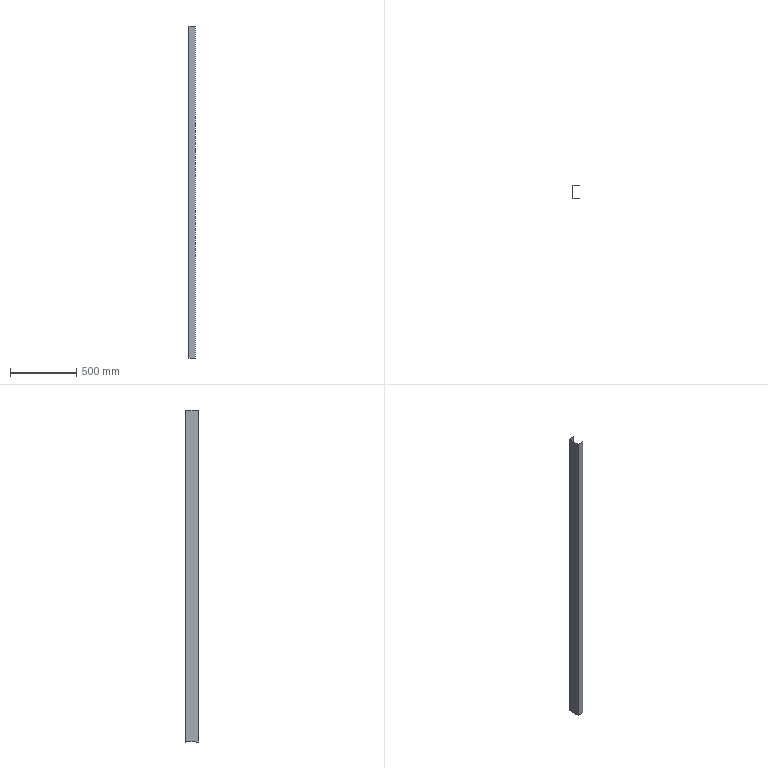Part | SolidWorks | features EdgeFlange 1, FlatPattern 1, SMBaseFlange 1, SheetMetal 1 | 1 solid | 22 faces | box 50 x 100 x 2500 mm | volume 733965 mm3 | plane 18 | cylinder 4 | commonest cylinder face diameters 1.473 x2 4.473 x2
STEP:
#1=CARTESIAN_POINT('',(-1.5,-47.763,-1250.));
#2=VERTEX_POINT('',#1);
#3=CARTESIAN_POINT('',(-1.5,-47.763,1250.));
#4=VERTEX_POINT('',#3);
#5=CARTESIAN_POINT('',(-1.5,-47.763,-1250.));
#6=DIRECTION('',(0.,0.,1.));
#7=VECTOR('',#6,1000.);
#8=LINE('',#5,#7);
#9=EDGE_CURVE('',#2,#4,#8,.T.);
#10=ORIENTED_EDGE('',*,*,#9,.T.);
#11=CARTESIAN_POINT('',(-1.5,47.763,1250.));
#12=VERTEX_POINT('',#11);
#13=CARTESIAN_POINT('',(-1.5,50.,1250.));
#14=DIRECTION('',(0.,-1.,0.));
#15=VECTOR('',#14,1000.);
#16=LINE('',#13,#15);
#17=EDGE_CURVE('',#12,#4,#16,.T.);
#18=ORIENTED_EDGE('',*,*,#17,.F.);
#19=CARTESIAN_POINT('',(-1.5,47.763,-1250.));
#20=VERTEX_POINT('',#19);
#21=CARTESIAN_POINT('',(-1.5,47.763,1250.));
#22=DIRECTION('',(0.,0.,-1.));
#23=VECTOR('',#22,1000.);
#24=LINE('',#21,#23);
#25=EDGE_CURVE('',#12,#20,#24,.T.);
#26=ORIENTED_EDGE('',*,*,#25,.T.);
#27=CARTESIAN_POINT('',(-1.5,50.,-1250.));
#28=DIRECTION('',(0.,1.,0.));
#29=VECTOR('',#28,1000.);
#30=LINE('',#27,#29);
#31=EDGE_CURVE('',#2,#20,#30,.T.);
#32=ORIENTED_EDGE('',*,*,#31,.F.);
#33=EDGE_LOOP('',(#10,#18,#26,#32));
#34=FACE_OUTER_BOUND('',#33,.T.);
#35=CARTESIAN_POINT('',(-1.5,0.,0.));
#36=DIRECTION('',(1.,0.,0.));
#37=DIRECTION('',(0.,0.,-1.));
#38=AXIS2_PLACEMENT_3D('',#35,#36,#37);
#39=PLANE('',#38);
#40=ADVANCED_FACE('',(#34),#39,.F.);
#41=CARTESIAN_POINT('',(0.,47.763,1250.));
#42=VERTEX_POINT('',#41);
#43=CARTESIAN_POINT('',(0.,-47.763,1250.));
#44=VERTEX_POINT('',#43);
#45=CARTESIAN_POINT('',(0.,50.,1250.));
#46=DIRECTION('',(0.,-1.,0.));
#47=VECTOR('',#46,1000.);
#48=LINE('',#45,#47);
#49=EDGE_CURVE('',#42,#44,#48,.T.);
#50=ORIENTED_EDGE('',*,*,#49,.T.);
#51=CARTESIAN_POINT('',(0.,-47.763,-1250.));
#52=VERTEX_POINT('',#51);
#53=CARTESIAN_POINT('',(0.,-47.763,-1250.));
#54=DIRECTION('',(0.,0.,1.));
#55=VECTOR('',#54,1000.);
#56=LINE('',#53,#55);
#57=EDGE_CURVE('',#52,#44,#56,.T.);
#58=ORIENTED_EDGE('',*,*,#57,.F.);
#59=CARTESIAN_POINT('',(0.,47.763,-1250.));
#60=VERTEX_POINT('',#59);
#61=CARTESIAN_POINT('',(0.,50.,-1250.));
#62=DIRECTION('',(0.,1.,0.));
#63=VECTOR('',#62,1000.);
#64=LINE('',#61,#63);
#65=EDGE_CURVE('',#52,#60,#64,.T.);
#66=ORIENTED_EDGE('',*,*,#65,.T.);
#67=CARTESIAN_POINT('',(0.,47.763,1250.));
#68=DIRECTION('',(0.,0.,-1.));
#69=VECTOR('',#68,1000.);
#70=LINE('',#67,#69);
#71=EDGE_CURVE('',#42,#60,#70,.T.);
#72=ORIENTED_EDGE('',*,*,#71,.F.);
#73=EDGE_LOOP('',(#50,#58,#66,#72));
#74=FACE_OUTER_BOUND('',#73,.T.);
#75=CARTESIAN_POINT('',(0.,0.,0.));
#76=DIRECTION('',(1.,0.,0.));
#77=DIRECTION('',(0.,0.,-1.));
#78=AXIS2_PLACEMENT_3D('',#75,#76,#77);
#79=PLANE('',#78);
#80=ADVANCED_FACE('',(#74),#79,.T.);
#81=ORIENTED_EDGE('',*,*,#65,.F.);
#82=CARTESIAN_POINT('',(0.,-47.763,-1250.));
#83=DIRECTION('',(-1.,0.,0.));
#84=VECTOR('',#83,1000.);
#85=LINE('',#82,#84);
#86=EDGE_CURVE('',#52,#2,#85,.T.);
#87=ORIENTED_EDGE('',*,*,#86,.T.);
#88=ORIENTED_EDGE('',*,*,#31,.T.);
#89=CARTESIAN_POINT('',(0.,47.763,-1250.));
#90=DIRECTION('',(-1.,0.,0.));
#91=VECTOR('',#90,1000.);
#92=LINE('',#89,#91);
#93=EDGE_CURVE('',#60,#20,#92,.T.);
#94=ORIENTED_EDGE('',*,*,#93,.F.);
#95=EDGE_LOOP('',(#81,#87,#88,#94));
#96=FACE_OUTER_BOUND('',#95,.T.);
#97=CARTESIAN_POINT('',(-1.5,50.,-1250.));
#98=DIRECTION('',(0.,0.,-1.));
#99=DIRECTION('',(-1.,0.,0.));
#100=AXIS2_PLACEMENT_3D('',#97,#98,#99);
#101=PLANE('',#100);
#102=ADVANCED_FACE('',(#96),#101,.T.);
#103=CARTESIAN_POINT('',(0.,-47.763,1250.));
#104=DIRECTION('',(-1.,0.,0.));
#105=VECTOR('',#104,1000.);
#106=LINE('',#103,#105);
#107=EDGE_CURVE('',#44,#4,#106,.T.);
#108=ORIENTED_EDGE('',*,*,#107,.F.);
#109=ORIENTED_EDGE('',*,*,#49,.F.);
#110=CARTESIAN_POINT('',(0.,47.763,1250.));
#111=DIRECTION('',(-1.,0.,0.));
#112=VECTOR('',#111,1000.);
#113=LINE('',#110,#112);
#114=EDGE_CURVE('',#42,#12,#113,.T.);
#115=ORIENTED_EDGE('',*,*,#114,.T.);
#116=ORIENTED_EDGE('',*,*,#17,.T.);
#117=EDGE_LOOP('',(#108,#109,#115,#116));
#118=FACE_OUTER_BOUND('',#117,.T.);
#119=CARTESIAN_POINT('',(-1.5,50.,1250.));
#120=DIRECTION('',(0.,0.,1.));
#121=DIRECTION('',(1.,0.,0.));
#122=AXIS2_PLACEMENT_3D('',#119,#120,#121);
#123=PLANE('',#122);
#124=ADVANCED_FACE('',(#118),#123,.T.);
#125=CARTESIAN_POINT('',(0.7366,48.5,-1250.));
#126=VERTEX_POINT('',#125);
#127=CARTESIAN_POINT('',(0.7366,50.,-1250.));
#128=VERTEX_POINT('',#127);
#129=CARTESIAN_POINT('',(0.7366,50.,-1250.));
#130=DIRECTION('',(0.,1.,0.));
#131=VECTOR('',#130,1000.);
#132=LINE('',#129,#131);
#133=EDGE_CURVE('',#126,#128,#132,.T.);
#134=ORIENTED_EDGE('',*,*,#133,.F.);
#135=CARTESIAN_POINT('',(0.7366,47.763,-1250.));
#136=DIRECTION('',(0.,0.,-1.));
#137=DIRECTION('',(1.,0.,0.));
#138=AXIS2_PLACEMENT_3D('',#135,#136,#137);
#139=CIRCLE('',#138,0.7366);
#140=EDGE_CURVE('',#60,#126,#139,.T.);
#141=ORIENTED_EDGE('',*,*,#140,.F.);
#142=ORIENTED_EDGE('',*,*,#93,.T.);
#143=CARTESIAN_POINT('',(0.7366,47.763,-1250.));
#144=DIRECTION('',(0.,0.,-1.));
#145=DIRECTION('',(1.,0.,0.));
#146=AXIS2_PLACEMENT_3D('',#143,#144,#145);
#147=CIRCLE('',#146,2.237);
#148=EDGE_CURVE('',#20,#128,#147,.T.);
#149=ORIENTED_EDGE('',*,*,#148,.T.);
#150=EDGE_LOOP('',(#134,#141,#142,#149));
#151=FACE_OUTER_BOUND('',#150,.T.);
#152=CARTESIAN_POINT('',(0.7366,47.763,-1250.));
#153=DIRECTION('',(0.,0.,-1.));
#154=DIRECTION('',(-1.,0.,0.));
#155=AXIS2_PLACEMENT_3D('',#152,#153,#154);
#156=PLANE('',#155);
#157=ADVANCED_FACE('',(#151),#156,.T.);
#158=CARTESIAN_POINT('',(0.7366,48.5,1250.));
#159=VERTEX_POINT('',#158);
#160=CARTESIAN_POINT('',(0.7366,47.763,1250.));
#161=DIRECTION('',(0.,0.,1.));
#162=DIRECTION('',(1.,0.,0.));
#163=AXIS2_PLACEMENT_3D('',#160,#161,#162);
#164=CIRCLE('',#163,0.7366);
#165=EDGE_CURVE('',#159,#42,#164,.T.);
#166=ORIENTED_EDGE('',*,*,#165,.F.);
#167=CARTESIAN_POINT('',(0.7366,50.,1250.));
#168=VERTEX_POINT('',#167);
#169=CARTESIAN_POINT('',(0.7366,48.5,1250.));
#170=DIRECTION('',(0.,1.,0.));
#171=VECTOR('',#170,1000.);
#172=LINE('',#169,#171);
#173=EDGE_CURVE('',#159,#168,#172,.T.);
#174=ORIENTED_EDGE('',*,*,#173,.T.);
#175=CARTESIAN_POINT('',(0.7366,47.763,1250.));
#176=DIRECTION('',(0.,0.,1.));
#177=DIRECTION('',(1.,0.,0.));
#178=AXIS2_PLACEMENT_3D('',#175,#176,#177);
#179=CIRCLE('',#178,2.237);
#180=EDGE_CURVE('',#168,#12,#179,.T.);
#181=ORIENTED_EDGE('',*,*,#180,.T.);
#182=ORIENTED_EDGE('',*,*,#114,.F.);
#183=EDGE_LOOP('',(#166,#174,#181,#182));
#184=FACE_OUTER_BOUND('',#183,.T.);
#185=CARTESIAN_POINT('',(0.7366,47.763,1250.));
#186=DIRECTION('',(0.,0.,-1.));
#187=DIRECTION('',(-1.,0.,0.));
#188=AXIS2_PLACEMENT_3D('',#185,#186,#187);
#189=PLANE('',#188);
#190=ADVANCED_FACE('',(#184),#189,.F.);
#191=ORIENTED_EDGE('',*,*,#25,.F.);
#192=ORIENTED_EDGE('',*,*,#180,.F.);
#193=CARTESIAN_POINT('',(0.7366,50.,-1250.));
#194=DIRECTION('',(0.,0.,-1.));
#195=VECTOR('',#194,1000.);
#196=LINE('',#193,#195);
#197=EDGE_CURVE('',#168,#128,#196,.T.);
#198=ORIENTED_EDGE('',*,*,#197,.T.);
#199=ORIENTED_EDGE('',*,*,#148,.F.);
#200=EDGE_LOOP('',(#191,#192,#198,#199));
#201=FACE_OUTER_BOUND('',#200,.T.);
#202=CARTESIAN_POINT('',(0.7366,47.763,1250.));
#203=DIRECTION('',(0.,0.,1.));
#204=DIRECTION('',(0.,1.,0.));
#205=AXIS2_PLACEMENT_3D('',#202,#203,#204);
#206=CYLINDRICAL_SURFACE('',#205,2.237);
#207=ADVANCED_FACE('',(#201),#206,.T.);
#208=ORIENTED_EDGE('',*,*,#71,.T.);
#209=ORIENTED_EDGE('',*,*,#140,.T.);
#210=CARTESIAN_POINT('',(0.7366,48.5,-1250.));
#211=DIRECTION('',(0.,0.,1.));
#212=VECTOR('',#211,1000.);
#213=LINE('',#210,#212);
#214=EDGE_CURVE('',#126,#159,#213,.T.);
#215=ORIENTED_EDGE('',*,*,#214,.T.);
#216=ORIENTED_EDGE('',*,*,#165,.T.);
#217=EDGE_LOOP('',(#208,#209,#215,#216));
#218=FACE_OUTER_BOUND('',#217,.T.);
#219=CARTESIAN_POINT('',(0.7366,47.763,1250.));
#220=DIRECTION('',(0.,0.,1.));
#221=DIRECTION('',(0.,1.,0.));
#222=AXIS2_PLACEMENT_3D('',#219,#220,#221);
#223=CYLINDRICAL_SURFACE('',#222,0.7366);
#224=ADVANCED_FACE('',(#218),#223,.F.);
#225=ORIENTED_EDGE('',*,*,#173,.F.);
#226=CARTESIAN_POINT('',(48.5,48.5,1250.));
#227=VERTEX_POINT('',#226);
#228=CARTESIAN_POINT('',(48.5,48.5,1250.));
#229=DIRECTION('',(1.,0.,0.));
#230=VECTOR('',#229,1000.);
#231=LINE('',#228,#230);
#232=EDGE_CURVE('',#159,#227,#231,.T.);
#233=ORIENTED_EDGE('',*,*,#232,.T.);
#234=CARTESIAN_POINT('',(48.5,50.,1250.));
#235=VERTEX_POINT('',#234);
#236=CARTESIAN_POINT('',(48.5,50.,1250.));
#237=DIRECTION('',(0.,-1.,0.));
#238=VECTOR('',#237,1000.);
#239=LINE('',#236,#238);
#240=EDGE_CURVE('',#235,#227,#239,.T.);
#241=ORIENTED_EDGE('',*,*,#240,.F.);
#242=CARTESIAN_POINT('',(0.,50.,1250.));
#243=DIRECTION('',(1.,0.,0.));
#244=VECTOR('',#243,1000.);
#245=LINE('',#242,#244);
#246=EDGE_CURVE('',#168,#235,#245,.T.);
#247=ORIENTED_EDGE('',*,*,#246,.F.);
#248=EDGE_LOOP('',(#225,#233,#241,#247));
#249=FACE_OUTER_BOUND('',#248,.T.);
#250=CARTESIAN_POINT('',(48.5,50.,1250.));
#251=DIRECTION('',(0.,0.,-1.));
#252=DIRECTION('',(-1.,0.,0.));
#253=AXIS2_PLACEMENT_3D('',#250,#251,#252);
#254=PLANE('',#253);
#255=ADVANCED_FACE('',(#249),#254,.F.);
#256=ORIENTED_EDGE('',*,*,#133,.T.);
#257=CARTESIAN_POINT('',(48.5,50.,-1250.));
#258=VERTEX_POINT('',#257);
#259=CARTESIAN_POINT('',(0.,50.,-1250.));
#260=DIRECTION('',(-1.,0.,0.));
#261=VECTOR('',#260,1000.);
#262=LINE('',#259,#261);
#263=EDGE_CURVE('',#258,#128,#262,.T.);
#264=ORIENTED_EDGE('',*,*,#263,.F.);
#265=CARTESIAN_POINT('',(48.5,48.5,-1250.));
#266=VERTEX_POINT('',#265);
#267=CARTESIAN_POINT('',(48.5,50.,-1250.));
#268=DIRECTION('',(0.,-1.,0.));
#269=VECTOR('',#268,1000.);
#270=LINE('',#267,#269);
#271=EDGE_CURVE('',#258,#266,#270,.T.);
#272=ORIENTED_EDGE('',*,*,#271,.T.);
#273=CARTESIAN_POINT('',(0.,48.5,-1250.));
#274=DIRECTION('',(-1.,0.,0.));
#275=VECTOR('',#274,1000.);
#276=LINE('',#273,#275);
#277=EDGE_CURVE('',#266,#126,#276,.T.);
#278=ORIENTED_EDGE('',*,*,#277,.T.);
#279=EDGE_LOOP('',(#256,#264,#272,#278));
#280=FACE_OUTER_BOUND('',#279,.T.);
#281=CARTESIAN_POINT('',(0.,50.,-1250.));
#282=DIRECTION('',(0.,0.,1.));
#283=DIRECTION('',(1.,0.,0.));
#284=AXIS2_PLACEMENT_3D('',#281,#282,#283);
#285=PLANE('',#284);
#286=ADVANCED_FACE('',(#280),#285,.F.);
#287=ORIENTED_EDGE('',*,*,#197,.F.);
#288=ORIENTED_EDGE('',*,*,#246,.T.);
#289=CARTESIAN_POINT('',(48.5,50.,0.));
#290=DIRECTION('',(0.,0.,-1.));
#291=VECTOR('',#290,1000.);
#292=LINE('',#289,#291);
#293=EDGE_CURVE('',#235,#258,#292,.T.);
#294=ORIENTED_EDGE('',*,*,#293,.T.);
#295=ORIENTED_EDGE('',*,*,#263,.T.);
#296=EDGE_LOOP('',(#287,#288,#294,#295));
#297=FACE_OUTER_BOUND('',#296,.T.);
#298=CARTESIAN_POINT('',(0.,50.,0.));
#299=DIRECTION('',(0.,-1.,0.));
#300=DIRECTION('',(1.,0.,0.));
#301=AXIS2_PLACEMENT_3D('',#298,#299,#300);
#302=PLANE('',#301);
#303=ADVANCED_FACE('',(#297),#302,.F.);
#304=ORIENTED_EDGE('',*,*,#232,.F.);
#305=ORIENTED_EDGE('',*,*,#214,.F.);
#306=ORIENTED_EDGE('',*,*,#277,.F.);
#307=CARTESIAN_POINT('',(48.5,48.5,-1250.));
#308=DIRECTION('',(0.,0.,-1.));
#309=VECTOR('',#308,1000.);
#310=LINE('',#307,#309);
#311=EDGE_CURVE('',#227,#266,#310,.T.);
#312=ORIENTED_EDGE('',*,*,#311,.F.);
#313=EDGE_LOOP('',(#304,#305,#306,#312));
#314=FACE_OUTER_BOUND('',#313,.T.);
#315=CARTESIAN_POINT('',(0.,48.5,0.));
#316=DIRECTION('',(0.,-1.,0.));
#317=DIRECTION('',(1.,0.,0.));
#318=AXIS2_PLACEMENT_3D('',#315,#316,#317);
#319=PLANE('',#318);
#320=ADVANCED_FACE('',(#314),#319,.T.);
#321=ORIENTED_EDGE('',*,*,#311,.T.);
#322=ORIENTED_EDGE('',*,*,#271,.F.);
#323=ORIENTED_EDGE('',*,*,#293,.F.);
#324=ORIENTED_EDGE('',*,*,#240,.T.);
#325=EDGE_LOOP('',(#321,#322,#323,#324));
#326=FACE_OUTER_BOUND('',#325,.T.);
#327=CARTESIAN_POINT('',(48.5,50.,-1250.));
#328=DIRECTION('',(-1.,0.,0.));
#329=DIRECTION('',(0.,-1.,0.));
#330=AXIS2_PLACEMENT_3D('',#327,#328,#329);
#331=PLANE('',#330);
#332=ADVANCED_FACE('',(#326),#331,.F.);
#333=CARTESIAN_POINT('',(0.7366,-48.5,1250.));
#334=VERTEX_POINT('',#333);
#335=CARTESIAN_POINT('',(0.7366,-50.,1250.));
#336=VERTEX_POINT('',#335);
#337=CARTESIAN_POINT('',(0.7366,-50.,1250.));
#338=DIRECTION('',(0.,-1.,0.));
#339=VECTOR('',#338,1000.);
#340=LINE('',#337,#339);
#341=EDGE_CURVE('',#334,#336,#340,.T.);
#342=ORIENTED_EDGE('',*,*,#341,.F.);
#343=CARTESIAN_POINT('',(0.7366,-47.763,1250.));
#344=DIRECTION('',(0.,0.,1.));
#345=DIRECTION('',(-1.,0.,0.));
#346=AXIS2_PLACEMENT_3D('',#343,#344,#345);
#347=CIRCLE('',#346,0.7366);
#348=EDGE_CURVE('',#44,#334,#347,.T.);
#349=ORIENTED_EDGE('',*,*,#348,.F.);
#350=ORIENTED_EDGE('',*,*,#107,.T.);
#351=CARTESIAN_POINT('',(0.7366,-47.763,1250.));
#352=DIRECTION('',(0.,0.,1.));
#353=DIRECTION('',(-1.,0.,0.));
#354=AXIS2_PLACEMENT_3D('',#351,#352,#353);
#355=CIRCLE('',#354,2.237);
#356=EDGE_CURVE('',#4,#336,#355,.T.);
#357=ORIENTED_EDGE('',*,*,#356,.T.);
#358=EDGE_LOOP('',(#342,#349,#350,#357));
#359=FACE_OUTER_BOUND('',#358,.T.);
#360=CARTESIAN_POINT('',(0.7366,-47.763,1250.));
#361=DIRECTION('',(0.,0.,1.));
#362=DIRECTION('',(1.,0.,0.));
#363=AXIS2_PLACEMENT_3D('',#360,#361,#362);
#364=PLANE('',#363);
#365=ADVANCED_FACE('',(#359),#364,.T.);
#366=CARTESIAN_POINT('',(0.7366,-48.5,-1250.));
#367=VERTEX_POINT('',#366);
#368=CARTESIAN_POINT('',(0.7366,-47.763,-1250.));
#369=DIRECTION('',(0.,0.,-1.));
#370=DIRECTION('',(-1.,0.,0.));
#371=AXIS2_PLACEMENT_3D('',#368,#369,#370);
#372=CIRCLE('',#371,0.7366);
#373=EDGE_CURVE('',#367,#52,#372,.T.);
#374=ORIENTED_EDGE('',*,*,#373,.F.);
#375=CARTESIAN_POINT('',(0.7366,-50.,-1250.));
#376=VERTEX_POINT('',#375);
#377=CARTESIAN_POINT('',(0.7366,-48.5,-1250.));
#378=DIRECTION('',(0.,-1.,0.));
#379=VECTOR('',#378,1000.);
#380=LINE('',#377,#379);
#381=EDGE_CURVE('',#367,#376,#380,.T.);
#382=ORIENTED_EDGE('',*,*,#381,.T.);
#383=CARTESIAN_POINT('',(0.7366,-47.763,-1250.));
#384=DIRECTION('',(0.,0.,-1.));
#385=DIRECTION('',(-1.,0.,0.));
#386=AXIS2_PLACEMENT_3D('',#383,#384,#385);
#387=CIRCLE('',#386,2.237);
#388=EDGE_CURVE('',#376,#2,#387,.T.);
#389=ORIENTED_EDGE('',*,*,#388,.T.);
#390=ORIENTED_EDGE('',*,*,#86,.F.);
#391=EDGE_LOOP('',(#374,#382,#389,#390));
#392=FACE_OUTER_BOUND('',#391,.T.);
#393=CARTESIAN_POINT('',(0.7366,-47.763,-1250.));
#394=DIRECTION('',(0.,0.,1.));
#395=DIRECTION('',(1.,0.,0.));
#396=AXIS2_PLACEMENT_3D('',#393,#394,#395);
#397=PLANE('',#396);
#398=ADVANCED_FACE('',(#392),#397,.F.);
#399=ORIENTED_EDGE('',*,*,#9,.F.);
#400=ORIENTED_EDGE('',*,*,#388,.F.);
#401=CARTESIAN_POINT('',(0.7366,-50.,1250.));
#402=DIRECTION('',(0.,0.,1.));
#403=VECTOR('',#402,1000.);
#404=LINE('',#401,#403);
#405=EDGE_CURVE('',#376,#336,#404,.T.);
#406=ORIENTED_EDGE('',*,*,#405,.T.);
#407=ORIENTED_EDGE('',*,*,#356,.F.);
#408=EDGE_LOOP('',(#399,#400,#406,#407));
#409=FACE_OUTER_BOUND('',#408,.T.);
#410=CARTESIAN_POINT('',(0.7366,-47.763,-1250.));
#411=DIRECTION('',(0.,0.,-1.));
#412=DIRECTION('',(0.,-1.,0.));
#413=AXIS2_PLACEMENT_3D('',#410,#411,#412);
#414=CYLINDRICAL_SURFACE('',#413,2.237);
#415=ADVANCED_FACE('',(#409),#414,.T.);
#416=ORIENTED_EDGE('',*,*,#57,.T.);
#417=ORIENTED_EDGE('',*,*,#348,.T.);
#418=CARTESIAN_POINT('',(0.7366,-48.5,1250.));
#419=DIRECTION('',(0.,0.,-1.));
#420=VECTOR('',#419,1000.);
#421=LINE('',#418,#420);
#422=EDGE_CURVE('',#334,#367,#421,.T.);
#423=ORIENTED_EDGE('',*,*,#422,.T.);
#424=ORIENTED_EDGE('',*,*,#373,.T.);
#425=EDGE_LOOP('',(#416,#417,#423,#424));
#426=FACE_OUTER_BOUND('',#425,.T.);
#427=CARTESIAN_POINT('',(0.7366,-47.763,-1250.));
#428=DIRECTION('',(0.,0.,-1.));
#429=DIRECTION('',(0.,-1.,0.));
#430=AXIS2_PLACEMENT_3D('',#427,#428,#429);
#431=CYLINDRICAL_SURFACE('',#430,0.7366);
#432=ADVANCED_FACE('',(#426),#431,.F.);
#433=ORIENTED_EDGE('',*,*,#341,.T.);
#434=CARTESIAN_POINT('',(48.5,-50.,1250.));
#435=VERTEX_POINT('',#434);
#436=CARTESIAN_POINT('',(0.,-50.,1250.));
#437=DIRECTION('',(-1.,0.,0.));
#438=VECTOR('',#437,1000.);
#439=LINE('',#436,#438);
#440=EDGE_CURVE('',#435,#336,#439,.T.);
#441=ORIENTED_EDGE('',*,*,#440,.F.);
#442=CARTESIAN_POINT('',(48.5,-48.5,1250.));
#443=VERTEX_POINT('',#442);
#444=CARTESIAN_POINT('',(48.5,-50.,1250.));
#445=DIRECTION('',(0.,1.,0.));
#446=VECTOR('',#445,1000.);
#447=LINE('',#444,#446);
#448=EDGE_CURVE('',#435,#443,#447,.T.);
#449=ORIENTED_EDGE('',*,*,#448,.T.);
#450=CARTESIAN_POINT('',(0.,-48.5,1250.));
#451=DIRECTION('',(-1.,0.,0.));
#452=VECTOR('',#451,1000.);
#453=LINE('',#450,#452);
#454=EDGE_CURVE('',#443,#334,#453,.T.);
#455=ORIENTED_EDGE('',*,*,#454,.T.);
#456=EDGE_LOOP('',(#433,#441,#449,#455));
#457=FACE_OUTER_BOUND('',#456,.T.);
#458=CARTESIAN_POINT('',(0.,-50.,1250.));
#459=DIRECTION('',(0.,0.,-1.));
#460=DIRECTION('',(-1.,0.,0.));
#461=AXIS2_PLACEMENT_3D('',#458,#459,#460);
#462=PLANE('',#461);
#463=ADVANCED_FACE('',(#457),#462,.F.);
#464=ORIENTED_EDGE('',*,*,#381,.F.);
#465=CARTESIAN_POINT('',(48.5,-48.5,-1250.));
#466=VERTEX_POINT('',#465);
#467=CARTESIAN_POINT('',(48.5,-48.5,-1250.));
#468=DIRECTION('',(1.,0.,0.));
#469=VECTOR('',#468,1000.);
#470=LINE('',#467,#469);
#471=EDGE_CURVE('',#367,#466,#470,.T.);
#472=ORIENTED_EDGE('',*,*,#471,.T.);
#473=CARTESIAN_POINT('',(48.5,-50.,-1250.));
#474=VERTEX_POINT('',#473);
#475=CARTESIAN_POINT('',(48.5,-50.,-1250.));
#476=DIRECTION('',(0.,1.,0.));
#477=VECTOR('',#476,1000.);
#478=LINE('',#475,#477);
#479=EDGE_CURVE('',#474,#466,#478,.T.);
#480=ORIENTED_EDGE('',*,*,#479,.F.);
#481=CARTESIAN_POINT('',(0.,-50.,-1250.));
#482=DIRECTION('',(1.,0.,0.));
#483=VECTOR('',#482,1000.);
#484=LINE('',#481,#483);
#485=EDGE_CURVE('',#376,#474,#484,.T.);
#486=ORIENTED_EDGE('',*,*,#485,.F.);
#487=EDGE_LOOP('',(#464,#472,#480,#486));
#488=FACE_OUTER_BOUND('',#487,.T.);
#489=CARTESIAN_POINT('',(48.5,-50.,-1250.));
#490=DIRECTION('',(0.,0.,1.));
#491=DIRECTION('',(1.,0.,0.));
#492=AXIS2_PLACEMENT_3D('',#489,#490,#491);
#493=PLANE('',#492);
#494=ADVANCED_FACE('',(#488),#493,.F.);
#495=ORIENTED_EDGE('',*,*,#405,.F.);
#496=ORIENTED_EDGE('',*,*,#485,.T.);
#497=CARTESIAN_POINT('',(48.5,-50.,0.));
#498=DIRECTION('',(0.,0.,1.));
#499=VECTOR('',#498,1000.);
#500=LINE('',#497,#499);
#501=EDGE_CURVE('',#474,#435,#500,.T.);
#502=ORIENTED_EDGE('',*,*,#501,.T.);
#503=ORIENTED_EDGE('',*,*,#440,.T.);
#504=EDGE_LOOP('',(#495,#496,#502,#503));
#505=FACE_OUTER_BOUND('',#504,.T.);
#506=CARTESIAN_POINT('',(0.,-50.,0.));
#507=DIRECTION('',(0.,1.,0.));
#508=DIRECTION('',(-1.,0.,0.));
#509=AXIS2_PLACEMENT_3D('',#506,#507,#508);
#510=PLANE('',#509);
#511=ADVANCED_FACE('',(#505),#510,.F.);
#512=ORIENTED_EDGE('',*,*,#471,.F.);
#513=ORIENTED_EDGE('',*,*,#422,.F.);
#514=ORIENTED_EDGE('',*,*,#454,.F.);
#515=CARTESIAN_POINT('',(48.5,-48.5,1250.));
#516=DIRECTION('',(0.,0.,1.));
#517=VECTOR('',#516,1000.);
#518=LINE('',#515,#517);
#519=EDGE_CURVE('',#466,#443,#518,.T.);
#520=ORIENTED_EDGE('',*,*,#519,.F.);
#521=EDGE_LOOP('',(#512,#513,#514,#520));
#522=FACE_OUTER_BOUND('',#521,.T.);
#523=CARTESIAN_POINT('',(0.,-48.5,0.));
#524=DIRECTION('',(0.,1.,0.));
#525=DIRECTION('',(-1.,0.,0.));
#526=AXIS2_PLACEMENT_3D('',#523,#524,#525);
#527=PLANE('',#526);
#528=ADVANCED_FACE('',(#522),#527,.T.);
#529=ORIENTED_EDGE('',*,*,#519,.T.);
#530=ORIENTED_EDGE('',*,*,#448,.F.);
#531=ORIENTED_EDGE('',*,*,#501,.F.);
#532=ORIENTED_EDGE('',*,*,#479,.T.);
#533=EDGE_LOOP('',(#529,#530,#531,#532));
#534=FACE_OUTER_BOUND('',#533,.T.);
#535=CARTESIAN_POINT('',(48.5,-50.,1250.));
#536=DIRECTION('',(-1.,0.,0.));
#537=DIRECTION('',(0.,-1.,0.));
#538=AXIS2_PLACEMENT_3D('',#535,#536,#537);
#539=PLANE('',#538);
#540=ADVANCED_FACE('',(#534),#539,.F.);
#541=CLOSED_SHELL('',(#40,#80,#102,#124,#157,#190,#207,#224,#255,#286,#303,#320,#332,#365,#398,#415,#432,#463,#494,#511,#528,#540));
#542=MANIFOLD_SOLID_BREP('',#541);
#543=CARTESIAN_POINT('',(0.,0.,0.));
#544=DIRECTION('',(0.,0.,1.));
#545=DIRECTION('',(1.,0.,0.));
#546=AXIS2_PLACEMENT_3D('',#543,#544,#545);
#547=(LENGTH_UNIT()NAMED_UNIT(*)SI_UNIT(.MILLI.,.METRE.));
#548=UNCERTAINTY_MEASURE_WITH_UNIT(LENGTH_MEASURE(0.00001),#547,'','');
#549=(NAMED_UNIT(*)PLANE_ANGLE_UNIT()SI_UNIT($,.RADIAN.));
#550=(NAMED_UNIT(*)SI_UNIT($,.STERADIAN.)SOLID_ANGLE_UNIT());
#551=(GEOMETRIC_REPRESENTATION_CONTEXT(3)GLOBAL_UNCERTAINTY_ASSIGNED_CONTEXT((#548))GLOBAL_UNIT_ASSIGNED_CONTEXT((#547,#549,#550))REPRESENTATION_CONTEXT('',''));
#552=ADVANCED_BREP_SHAPE_REPRESENTATION('',(#542,#546),#551);